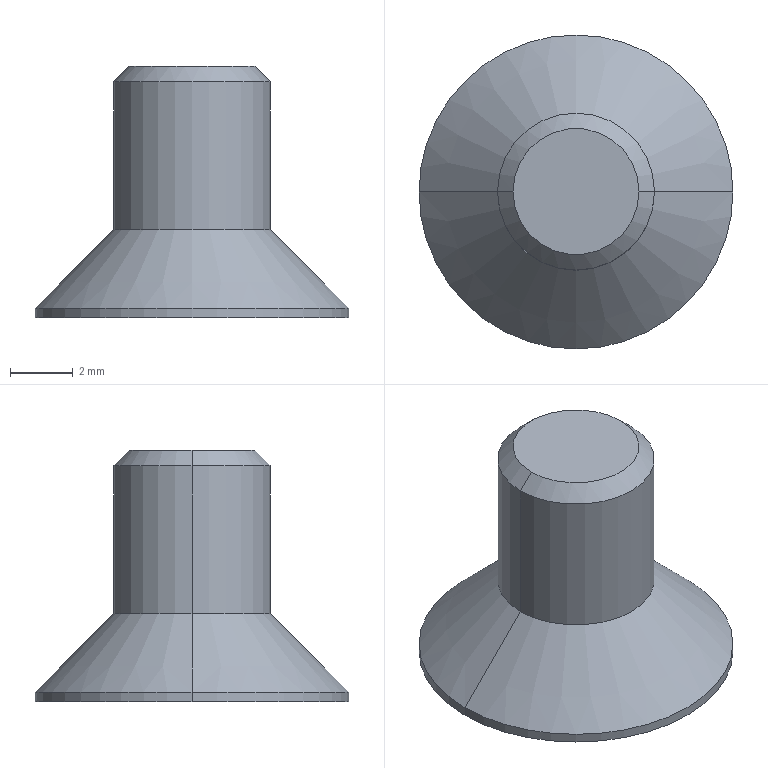Part | STEP file | 15 | 1 solid | 18 faces | box 10 x 10 x 8 mm | volume 218.465 mm3 | plane 8 | cone 6 | cylinder 4 | commonest cylinder face diameters 5 x2 10 x2